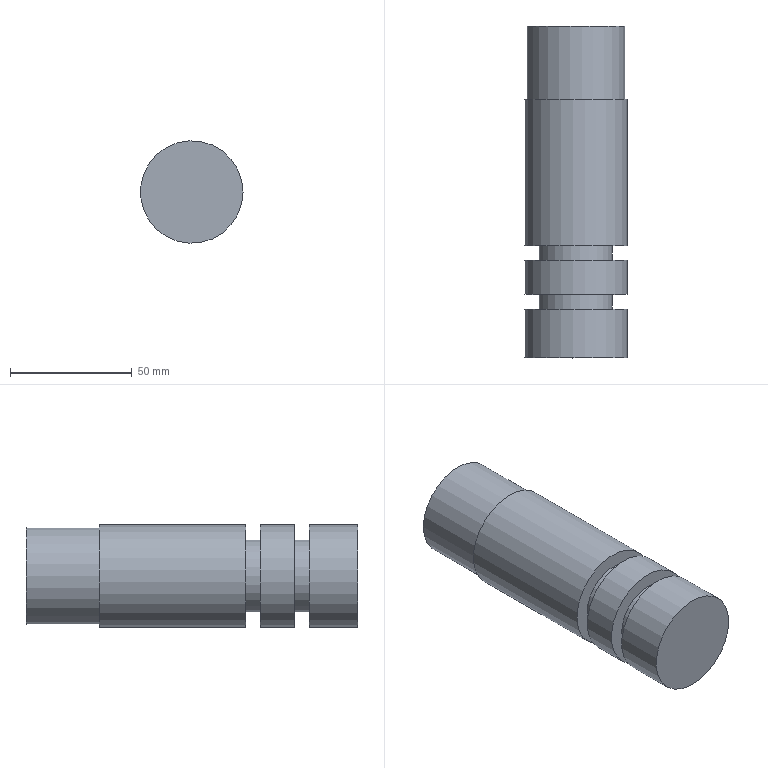Part | NX | features solid 2 | 1 solid | 13 faces | box 42 x 136 x 42 mm | volume 176413 mm3 | plane 7 | cylinder 6 | commonest cylinder face diameters 42 x3 30 x2 40 x1
STEP:
#1=CARTESIAN_POINT('',(511.,-435.,220.));
#2=VERTEX_POINT('',#1);
#3=CARTESIAN_POINT('',(490.,-435.,220.));
#4=DIRECTION('',(0.,-1.,0.));
#5=DIRECTION('',(1.,0.,0.));
#6=AXIS2_PLACEMENT_3D('',#3,#4,#5);
#7=CIRCLE('',#6,21.);
#8=EDGE_CURVE('',#2,#2,#7,.T.);
#9=ORIENTED_EDGE('',*,*,#8,.T.);
#10=EDGE_LOOP('',(#9));
#11=FACE_BOUND('',#10,.T.);
#12=CARTESIAN_POINT('',(505.,-435.,220.));
#13=VERTEX_POINT('',#12);
#14=CARTESIAN_POINT('',(490.,-435.,220.));
#15=DIRECTION('',(0.,-1.,0.));
#16=DIRECTION('',(1.,0.,0.));
#17=AXIS2_PLACEMENT_3D('',#14,#15,#16);
#18=CIRCLE('',#17,15.);
#19=EDGE_CURVE('',#13,#13,#18,.T.);
#20=ORIENTED_EDGE('',*,*,#19,.F.);
#21=EDGE_LOOP('',(#20));
#22=FACE_BOUND('',#21,.T.);
#23=CARTESIAN_POINT('',(490.,-435.,220.));
#24=DIRECTION('',(0.,-1.,0.));
#25=DIRECTION('',(0.,0.,-1.));
#26=AXIS2_PLACEMENT_3D('',#23,#24,#25);
#27=PLANE('',#26);
#28=ADVANCED_FACE('',(#11,#22),#27,.T.);
#29=CARTESIAN_POINT('',(511.,-415.,220.));
#30=VERTEX_POINT('',#29);
#31=CARTESIAN_POINT('',(490.,-415.,220.));
#32=DIRECTION('',(0.,-1.,0.));
#33=DIRECTION('',(1.,0.,0.));
#34=AXIS2_PLACEMENT_3D('',#31,#32,#33);
#35=CIRCLE('',#34,21.);
#36=EDGE_CURVE('',#30,#30,#35,.T.);
#37=ORIENTED_EDGE('',*,*,#36,.T.);
#38=EDGE_LOOP('',(#37));
#39=FACE_BOUND('',#38,.T.);
#40=CARTESIAN_POINT('',(505.,-415.,220.));
#41=VERTEX_POINT('',#40);
#42=CARTESIAN_POINT('',(490.,-415.,220.));
#43=DIRECTION('',(0.,-1.,0.));
#44=DIRECTION('',(1.,0.,0.));
#45=AXIS2_PLACEMENT_3D('',#42,#43,#44);
#46=CIRCLE('',#45,15.);
#47=EDGE_CURVE('',#41,#41,#46,.T.);
#48=ORIENTED_EDGE('',*,*,#47,.F.);
#49=EDGE_LOOP('',(#48));
#50=FACE_BOUND('',#49,.T.);
#51=CARTESIAN_POINT('',(490.,-415.,220.));
#52=DIRECTION('',(0.,-1.,0.));
#53=DIRECTION('',(0.,0.,-1.));
#54=AXIS2_PLACEMENT_3D('',#51,#52,#53);
#55=PLANE('',#54);
#56=ADVANCED_FACE('',(#39,#50),#55,.T.);
#57=ORIENTED_EDGE('',*,*,#36,.F.);
#58=EDGE_LOOP('',(#57));
#59=FACE_BOUND('',#58,.T.);
#60=CARTESIAN_POINT('',(511.,-355.,220.));
#61=VERTEX_POINT('',#60);
#62=CARTESIAN_POINT('',(490.,-355.,220.));
#63=DIRECTION('',(0.,-1.,0.));
#64=DIRECTION('',(1.,0.,0.));
#65=AXIS2_PLACEMENT_3D('',#62,#63,#64);
#66=CIRCLE('',#65,21.);
#67=EDGE_CURVE('',#61,#61,#66,.T.);
#68=ORIENTED_EDGE('',*,*,#67,.T.);
#69=EDGE_LOOP('',(#68));
#70=FACE_BOUND('',#69,.T.);
#71=CARTESIAN_POINT('',(490.,-415.,220.));
#72=DIRECTION('',(0.,1.,0.));
#73=DIRECTION('',(0.,0.,1.));
#74=AXIS2_PLACEMENT_3D('',#71,#72,#73);
#75=CYLINDRICAL_SURFACE('',#74,21.);
#76=ADVANCED_FACE('',(#59,#70),#75,.T.);
#77=CARTESIAN_POINT('',(510.,-355.,220.));
#78=VERTEX_POINT('',#77);
#79=CARTESIAN_POINT('',(490.,-355.,220.));
#80=DIRECTION('',(0.,-1.,0.));
#81=DIRECTION('',(1.,0.,0.));
#82=AXIS2_PLACEMENT_3D('',#79,#80,#81);
#83=CIRCLE('',#82,20.);
#84=EDGE_CURVE('',#78,#78,#83,.T.);
#85=ORIENTED_EDGE('',*,*,#84,.T.);
#86=EDGE_LOOP('',(#85));
#87=FACE_BOUND('',#86,.T.);
#88=ORIENTED_EDGE('',*,*,#67,.F.);
#89=EDGE_LOOP('',(#88));
#90=FACE_BOUND('',#89,.T.);
#91=CARTESIAN_POINT('',(490.,-355.,220.));
#92=DIRECTION('',(0.,-1.,0.));
#93=DIRECTION('',(0.,0.,-1.));
#94=AXIS2_PLACEMENT_3D('',#91,#92,#93);
#95=PLANE('',#94);
#96=ADVANCED_FACE('',(#87,#90),#95,.F.);
#97=CARTESIAN_POINT('',(510.,-325.,220.));
#98=VERTEX_POINT('',#97);
#99=CARTESIAN_POINT('',(490.,-325.,220.));
#100=DIRECTION('',(0.,-1.,0.));
#101=DIRECTION('',(1.,0.,0.));
#102=AXIS2_PLACEMENT_3D('',#99,#100,#101);
#103=CIRCLE('',#102,20.);
#104=EDGE_CURVE('',#98,#98,#103,.T.);
#105=ORIENTED_EDGE('',*,*,#104,.T.);
#106=EDGE_LOOP('',(#105));
#107=FACE_BOUND('',#106,.T.);
#108=ORIENTED_EDGE('',*,*,#84,.F.);
#109=EDGE_LOOP('',(#108));
#110=FACE_BOUND('',#109,.T.);
#111=CARTESIAN_POINT('',(490.,-325.,220.));
#112=DIRECTION('',(0.,-1.,0.));
#113=DIRECTION('',(0.,0.,-1.));
#114=AXIS2_PLACEMENT_3D('',#111,#112,#113);
#115=CYLINDRICAL_SURFACE('',#114,20.);
#116=ADVANCED_FACE('',(#107,#110),#115,.T.);
#117=ORIENTED_EDGE('',*,*,#104,.F.);
#118=EDGE_LOOP('',(#117));
#119=FACE_BOUND('',#118,.T.);
#120=CARTESIAN_POINT('',(490.,-325.,220.));
#121=DIRECTION('',(0.,-1.,0.));
#122=DIRECTION('',(0.,0.,-1.));
#123=AXIS2_PLACEMENT_3D('',#120,#121,#122);
#124=PLANE('',#123);
#125=ADVANCED_FACE('',(#119),#124,.F.);
#126=CARTESIAN_POINT('',(505.,-421.,220.));
#127=VERTEX_POINT('',#126);
#128=CARTESIAN_POINT('',(490.,-421.,220.));
#129=DIRECTION('',(0.,-1.,0.));
#130=DIRECTION('',(1.,0.,0.));
#131=AXIS2_PLACEMENT_3D('',#128,#129,#130);
#132=CIRCLE('',#131,15.);
#133=EDGE_CURVE('',#127,#127,#132,.T.);
#134=ORIENTED_EDGE('',*,*,#133,.F.);
#135=EDGE_LOOP('',(#134));
#136=FACE_BOUND('',#135,.T.);
#137=ORIENTED_EDGE('',*,*,#47,.T.);
#138=EDGE_LOOP('',(#137));
#139=FACE_BOUND('',#138,.T.);
#140=CARTESIAN_POINT('',(490.,-421.,220.));
#141=DIRECTION('',(0.,1.,0.));
#142=DIRECTION('',(0.,0.,1.));
#143=AXIS2_PLACEMENT_3D('',#140,#141,#142);
#144=CYLINDRICAL_SURFACE('',#143,15.);
#145=ADVANCED_FACE('',(#136,#139),#144,.T.);
#146=CARTESIAN_POINT('',(511.,-421.,220.));
#147=VERTEX_POINT('',#146);
#148=CARTESIAN_POINT('',(490.,-421.,220.));
#149=DIRECTION('',(0.,-1.,0.));
#150=DIRECTION('',(1.,0.,0.));
#151=AXIS2_PLACEMENT_3D('',#148,#149,#150);
#152=CIRCLE('',#151,21.);
#153=EDGE_CURVE('',#147,#147,#152,.T.);
#154=ORIENTED_EDGE('',*,*,#153,.F.);
#155=EDGE_LOOP('',(#154));
#156=FACE_BOUND('',#155,.T.);
#157=ORIENTED_EDGE('',*,*,#133,.T.);
#158=EDGE_LOOP('',(#157));
#159=FACE_BOUND('',#158,.T.);
#160=CARTESIAN_POINT('',(490.,-421.,220.));
#161=DIRECTION('',(0.,-1.,0.));
#162=DIRECTION('',(0.,0.,-1.));
#163=AXIS2_PLACEMENT_3D('',#160,#161,#162);
#164=PLANE('',#163);
#165=ADVANCED_FACE('',(#156,#159),#164,.F.);
#166=ORIENTED_EDGE('',*,*,#8,.F.);
#167=EDGE_LOOP('',(#166));
#168=FACE_BOUND('',#167,.T.);
#169=ORIENTED_EDGE('',*,*,#153,.T.);
#170=EDGE_LOOP('',(#169));
#171=FACE_BOUND('',#170,.T.);
#172=CARTESIAN_POINT('',(490.,-435.,220.));
#173=DIRECTION('',(0.,1.,0.));
#174=DIRECTION('',(0.,0.,1.));
#175=AXIS2_PLACEMENT_3D('',#172,#173,#174);
#176=CYLINDRICAL_SURFACE('',#175,21.);
#177=ADVANCED_FACE('',(#168,#171),#176,.T.);
#178=CARTESIAN_POINT('',(505.,-441.,220.));
#179=VERTEX_POINT('',#178);
#180=CARTESIAN_POINT('',(490.,-441.,220.));
#181=DIRECTION('',(0.,-1.,0.));
#182=DIRECTION('',(1.,0.,0.));
#183=AXIS2_PLACEMENT_3D('',#180,#181,#182);
#184=CIRCLE('',#183,15.);
#185=EDGE_CURVE('',#179,#179,#184,.T.);
#186=ORIENTED_EDGE('',*,*,#185,.F.);
#187=EDGE_LOOP('',(#186));
#188=FACE_BOUND('',#187,.T.);
#189=ORIENTED_EDGE('',*,*,#19,.T.);
#190=EDGE_LOOP('',(#189));
#191=FACE_BOUND('',#190,.T.);
#192=CARTESIAN_POINT('',(490.,-441.,220.));
#193=DIRECTION('',(0.,1.,0.));
#194=DIRECTION('',(0.,0.,1.));
#195=AXIS2_PLACEMENT_3D('',#192,#193,#194);
#196=CYLINDRICAL_SURFACE('',#195,15.);
#197=ADVANCED_FACE('',(#188,#191),#196,.T.);
#198=CARTESIAN_POINT('',(511.,-441.,220.));
#199=VERTEX_POINT('',#198);
#200=CARTESIAN_POINT('',(490.,-441.,220.));
#201=DIRECTION('',(0.,-1.,0.));
#202=DIRECTION('',(1.,0.,0.));
#203=AXIS2_PLACEMENT_3D('',#200,#201,#202);
#204=CIRCLE('',#203,21.);
#205=EDGE_CURVE('',#199,#199,#204,.T.);
#206=ORIENTED_EDGE('',*,*,#205,.F.);
#207=EDGE_LOOP('',(#206));
#208=FACE_BOUND('',#207,.T.);
#209=ORIENTED_EDGE('',*,*,#185,.T.);
#210=EDGE_LOOP('',(#209));
#211=FACE_BOUND('',#210,.T.);
#212=CARTESIAN_POINT('',(490.,-441.,220.));
#213=DIRECTION('',(0.,-1.,0.));
#214=DIRECTION('',(0.,0.,-1.));
#215=AXIS2_PLACEMENT_3D('',#212,#213,#214);
#216=PLANE('',#215);
#217=ADVANCED_FACE('',(#208,#211),#216,.F.);
#218=CARTESIAN_POINT('',(511.,-461.,220.));
#219=VERTEX_POINT('',#218);
#220=CARTESIAN_POINT('',(490.,-461.,220.));
#221=DIRECTION('',(0.,-1.,0.));
#222=DIRECTION('',(1.,0.,0.));
#223=AXIS2_PLACEMENT_3D('',#220,#221,#222);
#224=CIRCLE('',#223,21.);
#225=EDGE_CURVE('',#219,#219,#224,.T.);
#226=ORIENTED_EDGE('',*,*,#225,.F.);
#227=EDGE_LOOP('',(#226));
#228=FACE_BOUND('',#227,.T.);
#229=ORIENTED_EDGE('',*,*,#205,.T.);
#230=EDGE_LOOP('',(#229));
#231=FACE_BOUND('',#230,.T.);
#232=CARTESIAN_POINT('',(490.,-461.,220.));
#233=DIRECTION('',(0.,1.,0.));
#234=DIRECTION('',(0.,0.,1.));
#235=AXIS2_PLACEMENT_3D('',#232,#233,#234);
#236=CYLINDRICAL_SURFACE('',#235,21.);
#237=ADVANCED_FACE('',(#228,#231),#236,.T.);
#238=ORIENTED_EDGE('',*,*,#225,.T.);
#239=EDGE_LOOP('',(#238));
#240=FACE_BOUND('',#239,.T.);
#241=CARTESIAN_POINT('',(490.,-461.,220.));
#242=DIRECTION('',(0.,-1.,0.));
#243=DIRECTION('',(0.,0.,-1.));
#244=AXIS2_PLACEMENT_3D('',#241,#242,#243);
#245=PLANE('',#244);
#246=ADVANCED_FACE('',(#240),#245,.T.);
#247=CLOSED_SHELL('',(#28,#56,#76,#96,#116,#125,#145,#165,#177,#197,#217,#237,#246));
#248=MANIFOLD_SOLID_BREP('',#247);
#249=(LENGTH_UNIT()NAMED_UNIT(*)SI_UNIT(.MILLI.,.METRE.));
#250=UNCERTAINTY_MEASURE_WITH_UNIT(LENGTH_MEASURE(0.00001),#249,'','');
#251=(NAMED_UNIT(*)PLANE_ANGLE_UNIT()SI_UNIT($,.RADIAN.));
#252=(NAMED_UNIT(*)SI_UNIT($,.STERADIAN.)SOLID_ANGLE_UNIT());
#253=(GEOMETRIC_REPRESENTATION_CONTEXT(3)GLOBAL_UNCERTAINTY_ASSIGNED_CONTEXT((#250))GLOBAL_UNIT_ASSIGNED_CONTEXT((#249,#251,#252))REPRESENTATION_CONTEXT('',''));
#254=ADVANCED_BREP_SHAPE_REPRESENTATION('',(#248),#253);